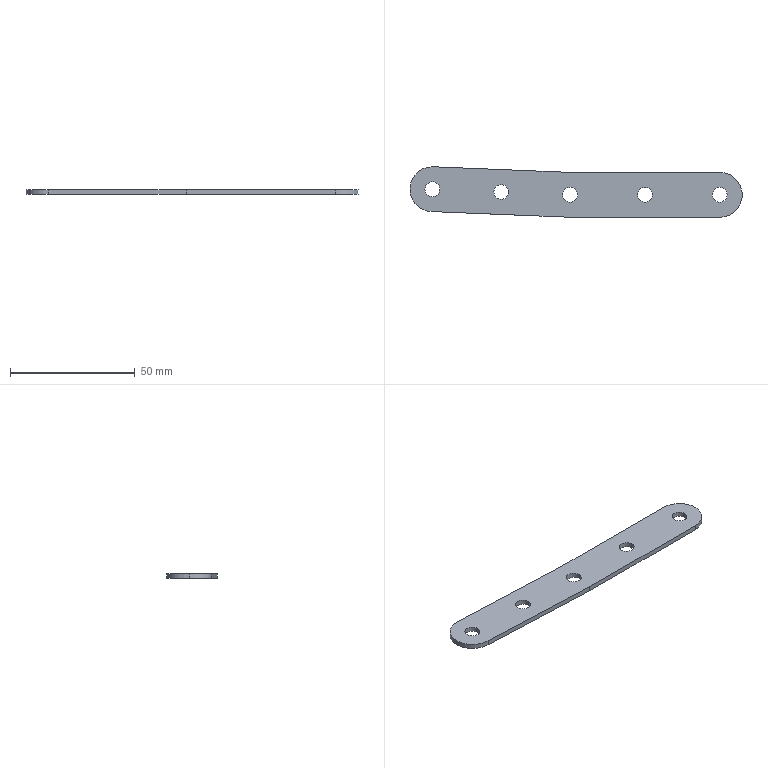Part | SolidWorks | features Extrusion 1 | 1 solid | 19 faces | box 133.234 x 20.271 x 2 mm | volume 4375 mm3 | cylinder 13 | plane 6 | commonest cylinder face diameters 6 x10 18 x3
STEP:
#1=CARTESIAN_POINT('',(82.234,-2.271,2.));
#2=VERTEX_POINT('',#1);
#3=CARTESIAN_POINT('',(88.234,-2.271,2.));
#4=VERTEX_POINT('',#3);
#5=CARTESIAN_POINT('',(85.234,-2.271,2.));
#6=DIRECTION('',(0.,0.,1.));
#7=DIRECTION('',(1.,0.,0.));
#8=AXIS2_PLACEMENT_3D('',#5,#6,#7);
#9=CIRCLE('',#8,3.);
#10=EDGE_CURVE('',#2,#4,#9,.T.);
#11=ORIENTED_EDGE('',*,*,#10,.T.);
#12=CARTESIAN_POINT('',(88.234,-2.271,0.));
#13=VERTEX_POINT('',#12);
#14=CARTESIAN_POINT('',(88.234,-2.271,2.));
#15=DIRECTION('',(0.,0.,-1.));
#16=VECTOR('',#15,1000.);
#17=LINE('',#14,#16);
#18=EDGE_CURVE('',#4,#13,#17,.T.);
#19=ORIENTED_EDGE('',*,*,#18,.T.);
#20=CARTESIAN_POINT('',(82.234,-2.271,0.));
#21=VERTEX_POINT('',#20);
#22=CARTESIAN_POINT('',(85.234,-2.271,0.));
#23=DIRECTION('',(0.,0.,1.));
#24=DIRECTION('',(1.,0.,0.));
#25=AXIS2_PLACEMENT_3D('',#22,#23,#24);
#26=CIRCLE('',#25,3.);
#27=EDGE_CURVE('',#21,#13,#26,.T.);
#28=ORIENTED_EDGE('',*,*,#27,.F.);
#29=CARTESIAN_POINT('',(82.234,-2.271,2.));
#30=DIRECTION('',(0.,0.,-1.));
#31=VECTOR('',#30,1000.);
#32=LINE('',#29,#31);
#33=EDGE_CURVE('',#2,#21,#32,.T.);
#34=ORIENTED_EDGE('',*,*,#33,.F.);
#35=EDGE_LOOP('',(#11,#19,#28,#34));
#36=FACE_OUTER_BOUND('',#35,.T.);
#37=CARTESIAN_POINT('',(85.234,-2.271,2.));
#38=DIRECTION('',(0.,0.,-1.));
#39=DIRECTION('',(-1.,0.,0.));
#40=AXIS2_PLACEMENT_3D('',#37,#38,#39);
#41=CYLINDRICAL_SURFACE('',#40,3.);
#42=ADVANCED_FACE('',(#36),#41,.F.);
#43=CARTESIAN_POINT('',(24.617,-1.136,2.));
#44=VERTEX_POINT('',#43);
#45=CARTESIAN_POINT('',(30.617,-1.136,2.));
#46=VERTEX_POINT('',#45);
#47=CARTESIAN_POINT('',(27.617,-1.136,2.));
#48=DIRECTION('',(0.,0.,1.));
#49=DIRECTION('',(1.,0.,0.));
#50=AXIS2_PLACEMENT_3D('',#47,#48,#49);
#51=CIRCLE('',#50,3.);
#52=EDGE_CURVE('',#44,#46,#51,.T.);
#53=ORIENTED_EDGE('',*,*,#52,.T.);
#54=CARTESIAN_POINT('',(30.617,-1.136,0.));
#55=VERTEX_POINT('',#54);
#56=CARTESIAN_POINT('',(30.617,-1.136,2.));
#57=DIRECTION('',(0.,0.,-1.));
#58=VECTOR('',#57,1000.);
#59=LINE('',#56,#58);
#60=EDGE_CURVE('',#46,#55,#59,.T.);
#61=ORIENTED_EDGE('',*,*,#60,.T.);
#62=CARTESIAN_POINT('',(24.617,-1.136,0.));
#63=VERTEX_POINT('',#62);
#64=CARTESIAN_POINT('',(27.617,-1.136,0.));
#65=DIRECTION('',(0.,0.,1.));
#66=DIRECTION('',(1.,0.,0.));
#67=AXIS2_PLACEMENT_3D('',#64,#65,#66);
#68=CIRCLE('',#67,3.);
#69=EDGE_CURVE('',#63,#55,#68,.T.);
#70=ORIENTED_EDGE('',*,*,#69,.F.);
#71=CARTESIAN_POINT('',(24.617,-1.136,2.));
#72=DIRECTION('',(0.,0.,-1.));
#73=VECTOR('',#72,1000.);
#74=LINE('',#71,#73);
#75=EDGE_CURVE('',#44,#63,#74,.T.);
#76=ORIENTED_EDGE('',*,*,#75,.F.);
#77=EDGE_LOOP('',(#53,#61,#70,#76));
#78=FACE_OUTER_BOUND('',#77,.T.);
#79=CARTESIAN_POINT('',(27.617,-1.136,2.));
#80=DIRECTION('',(0.,0.,-1.));
#81=DIRECTION('',(-1.,0.,0.));
#82=AXIS2_PLACEMENT_3D('',#79,#80,#81);
#83=CYLINDRICAL_SURFACE('',#82,3.);
#84=ADVANCED_FACE('',(#78),#83,.F.);
#85=CARTESIAN_POINT('',(112.234,-2.271,2.));
#86=VERTEX_POINT('',#85);
#87=CARTESIAN_POINT('',(118.234,-2.271,2.));
#88=VERTEX_POINT('',#87);
#89=CARTESIAN_POINT('',(115.234,-2.271,2.));
#90=DIRECTION('',(0.,0.,1.));
#91=DIRECTION('',(1.,0.,0.));
#92=AXIS2_PLACEMENT_3D('',#89,#90,#91);
#93=CIRCLE('',#92,3.);
#94=EDGE_CURVE('',#86,#88,#93,.T.);
#95=ORIENTED_EDGE('',*,*,#94,.T.);
#96=CARTESIAN_POINT('',(118.234,-2.271,0.));
#97=VERTEX_POINT('',#96);
#98=CARTESIAN_POINT('',(118.234,-2.271,2.));
#99=DIRECTION('',(0.,0.,-1.));
#100=VECTOR('',#99,1000.);
#101=LINE('',#98,#100);
#102=EDGE_CURVE('',#88,#97,#101,.T.);
#103=ORIENTED_EDGE('',*,*,#102,.T.);
#104=CARTESIAN_POINT('',(112.234,-2.271,0.));
#105=VERTEX_POINT('',#104);
#106=CARTESIAN_POINT('',(115.234,-2.271,0.));
#107=DIRECTION('',(0.,0.,1.));
#108=DIRECTION('',(1.,0.,0.));
#109=AXIS2_PLACEMENT_3D('',#106,#107,#108);
#110=CIRCLE('',#109,3.);
#111=EDGE_CURVE('',#105,#97,#110,.T.);
#112=ORIENTED_EDGE('',*,*,#111,.F.);
#113=CARTESIAN_POINT('',(112.234,-2.271,2.));
#114=DIRECTION('',(0.,0.,-1.));
#115=VECTOR('',#114,1000.);
#116=LINE('',#113,#115);
#117=EDGE_CURVE('',#86,#105,#116,.T.);
#118=ORIENTED_EDGE('',*,*,#117,.F.);
#119=EDGE_LOOP('',(#95,#103,#112,#118));
#120=FACE_OUTER_BOUND('',#119,.T.);
#121=CARTESIAN_POINT('',(115.234,-2.271,2.));
#122=DIRECTION('',(0.,0.,-1.));
#123=DIRECTION('',(-1.,0.,0.));
#124=AXIS2_PLACEMENT_3D('',#121,#122,#123);
#125=CYLINDRICAL_SURFACE('',#124,3.);
#126=ADVANCED_FACE('',(#120),#125,.F.);
#127=CARTESIAN_POINT('',(52.234,-2.271,2.));
#128=VERTEX_POINT('',#127);
#129=CARTESIAN_POINT('',(58.234,-2.271,2.));
#130=VERTEX_POINT('',#129);
#131=CARTESIAN_POINT('',(55.234,-2.271,2.));
#132=DIRECTION('',(0.,0.,1.));
#133=DIRECTION('',(1.,0.,0.));
#134=AXIS2_PLACEMENT_3D('',#131,#132,#133);
#135=CIRCLE('',#134,3.);
#136=EDGE_CURVE('',#128,#130,#135,.T.);
#137=ORIENTED_EDGE('',*,*,#136,.T.);
#138=CARTESIAN_POINT('',(58.234,-2.271,0.));
#139=VERTEX_POINT('',#138);
#140=CARTESIAN_POINT('',(58.234,-2.271,2.));
#141=DIRECTION('',(0.,0.,-1.));
#142=VECTOR('',#141,1000.);
#143=LINE('',#140,#142);
#144=EDGE_CURVE('',#130,#139,#143,.T.);
#145=ORIENTED_EDGE('',*,*,#144,.T.);
#146=CARTESIAN_POINT('',(52.234,-2.271,0.));
#147=VERTEX_POINT('',#146);
#148=CARTESIAN_POINT('',(55.234,-2.271,0.));
#149=DIRECTION('',(0.,0.,1.));
#150=DIRECTION('',(1.,0.,0.));
#151=AXIS2_PLACEMENT_3D('',#148,#149,#150);
#152=CIRCLE('',#151,3.);
#153=EDGE_CURVE('',#147,#139,#152,.T.);
#154=ORIENTED_EDGE('',*,*,#153,.F.);
#155=CARTESIAN_POINT('',(52.234,-2.271,2.));
#156=DIRECTION('',(0.,0.,-1.));
#157=VECTOR('',#156,1000.);
#158=LINE('',#155,#157);
#159=EDGE_CURVE('',#128,#147,#158,.T.);
#160=ORIENTED_EDGE('',*,*,#159,.F.);
#161=EDGE_LOOP('',(#137,#145,#154,#160));
#162=FACE_OUTER_BOUND('',#161,.T.);
#163=CARTESIAN_POINT('',(55.234,-2.271,2.));
#164=DIRECTION('',(0.,0.,-1.));
#165=DIRECTION('',(-1.,0.,0.));
#166=AXIS2_PLACEMENT_3D('',#163,#164,#165);
#167=CYLINDRICAL_SURFACE('',#166,3.);
#168=ADVANCED_FACE('',(#162),#167,.F.);
#169=CARTESIAN_POINT('',(-3.,0.,2.));
#170=VERTEX_POINT('',#169);
#171=CARTESIAN_POINT('',(3.,0.,2.));
#172=VERTEX_POINT('',#171);
#173=CARTESIAN_POINT('',(0.,0.,2.));
#174=DIRECTION('',(0.,0.,1.));
#175=DIRECTION('',(1.,0.,0.));
#176=AXIS2_PLACEMENT_3D('',#173,#174,#175);
#177=CIRCLE('',#176,3.);
#178=EDGE_CURVE('',#170,#172,#177,.T.);
#179=ORIENTED_EDGE('',*,*,#178,.T.);
#180=CARTESIAN_POINT('',(3.,0.,0.));
#181=VERTEX_POINT('',#180);
#182=CARTESIAN_POINT('',(3.,0.,2.));
#183=DIRECTION('',(0.,0.,-1.));
#184=VECTOR('',#183,1000.);
#185=LINE('',#182,#184);
#186=EDGE_CURVE('',#172,#181,#185,.T.);
#187=ORIENTED_EDGE('',*,*,#186,.T.);
#188=CARTESIAN_POINT('',(-3.,0.,0.));
#189=VERTEX_POINT('',#188);
#190=CARTESIAN_POINT('',(0.,0.,0.));
#191=DIRECTION('',(0.,0.,1.));
#192=DIRECTION('',(1.,0.,0.));
#193=AXIS2_PLACEMENT_3D('',#190,#191,#192);
#194=CIRCLE('',#193,3.);
#195=EDGE_CURVE('',#189,#181,#194,.T.);
#196=ORIENTED_EDGE('',*,*,#195,.F.);
#197=CARTESIAN_POINT('',(-3.,0.,2.));
#198=DIRECTION('',(0.,0.,-1.));
#199=VECTOR('',#198,1000.);
#200=LINE('',#197,#199);
#201=EDGE_CURVE('',#170,#189,#200,.T.);
#202=ORIENTED_EDGE('',*,*,#201,.F.);
#203=EDGE_LOOP('',(#179,#187,#196,#202));
#204=FACE_OUTER_BOUND('',#203,.T.);
#205=CARTESIAN_POINT('',(0.,0.,2.));
#206=DIRECTION('',(0.,0.,-1.));
#207=DIRECTION('',(-1.,0.,0.));
#208=AXIS2_PLACEMENT_3D('',#205,#206,#207);
#209=CYLINDRICAL_SURFACE('',#208,3.);
#210=ADVANCED_FACE('',(#204),#209,.F.);
#211=CARTESIAN_POINT('',(-9.,0.,2.));
#212=VERTEX_POINT('',#211);
#213=CARTESIAN_POINT('',(0.,-9.,2.));
#214=VERTEX_POINT('',#213);
#215=CARTESIAN_POINT('',(0.,0.,2.));
#216=DIRECTION('',(0.,0.,1.));
#217=DIRECTION('',(1.,0.,0.));
#218=AXIS2_PLACEMENT_3D('',#215,#216,#217);
#219=CIRCLE('',#218,9.);
#220=EDGE_CURVE('',#212,#214,#219,.T.);
#221=ORIENTED_EDGE('',*,*,#220,.F.);
#222=CARTESIAN_POINT('',(-9.,0.,0.));
#223=VERTEX_POINT('',#222);
#224=CARTESIAN_POINT('',(-9.,0.,2.));
#225=DIRECTION('',(0.,0.,-1.));
#226=VECTOR('',#225,1000.);
#227=LINE('',#224,#226);
#228=EDGE_CURVE('',#212,#223,#227,.T.);
#229=ORIENTED_EDGE('',*,*,#228,.T.);
#230=CARTESIAN_POINT('',(0.,-9.,0.));
#231=VERTEX_POINT('',#230);
#232=CARTESIAN_POINT('',(0.,0.,0.));
#233=DIRECTION('',(0.,0.,1.));
#234=DIRECTION('',(1.,0.,0.));
#235=AXIS2_PLACEMENT_3D('',#232,#233,#234);
#236=CIRCLE('',#235,9.);
#237=EDGE_CURVE('',#223,#231,#236,.T.);
#238=ORIENTED_EDGE('',*,*,#237,.T.);
#239=CARTESIAN_POINT('',(0.,-9.,2.));
#240=DIRECTION('',(0.,0.,-1.));
#241=VECTOR('',#240,1000.);
#242=LINE('',#239,#241);
#243=EDGE_CURVE('',#214,#231,#242,.T.);
#244=ORIENTED_EDGE('',*,*,#243,.F.);
#245=EDGE_LOOP('',(#221,#229,#238,#244));
#246=FACE_OUTER_BOUND('',#245,.T.);
#247=CARTESIAN_POINT('',(0.,0.,2.));
#248=DIRECTION('',(0.,0.,-1.));
#249=DIRECTION('',(-1.,0.,0.));
#250=AXIS2_PLACEMENT_3D('',#247,#248,#249);
#251=CYLINDRICAL_SURFACE('',#250,9.);
#252=ADVANCED_FACE('',(#246),#251,.T.);
#253=ORIENTED_EDGE('',*,*,#52,.F.);
#254=CARTESIAN_POINT('',(27.617,-1.136,2.));
#255=DIRECTION('',(0.,0.,1.));
#256=DIRECTION('',(1.,0.,0.));
#257=AXIS2_PLACEMENT_3D('',#254,#255,#256);
#258=CIRCLE('',#257,3.);
#259=EDGE_CURVE('',#46,#44,#258,.T.);
#260=ORIENTED_EDGE('',*,*,#259,.F.);
#261=EDGE_LOOP('',(#253,#260));
#262=FACE_BOUND('',#261,.T.);
#263=ORIENTED_EDGE('',*,*,#136,.F.);
#264=CARTESIAN_POINT('',(55.234,-2.271,2.));
#265=DIRECTION('',(0.,0.,1.));
#266=DIRECTION('',(1.,0.,0.));
#267=AXIS2_PLACEMENT_3D('',#264,#265,#266);
#268=CIRCLE('',#267,3.);
#269=EDGE_CURVE('',#130,#128,#268,.T.);
#270=ORIENTED_EDGE('',*,*,#269,.F.);
#271=EDGE_LOOP('',(#263,#270));
#272=FACE_BOUND('',#271,.T.);
#273=CARTESIAN_POINT('',(0.,9.,2.));
#274=VERTEX_POINT('',#273);
#275=CARTESIAN_POINT('',(0.,0.,2.));
#276=DIRECTION('',(0.,0.,1.));
#277=DIRECTION('',(1.,0.,0.));
#278=AXIS2_PLACEMENT_3D('',#275,#276,#277);
#279=CIRCLE('',#278,9.);
#280=EDGE_CURVE('',#274,#212,#279,.T.);
#281=ORIENTED_EDGE('',*,*,#280,.T.);
#282=ORIENTED_EDGE('',*,*,#220,.T.);
#283=CARTESIAN_POINT('',(55.234,-11.271,2.));
#284=VERTEX_POINT('',#283);
#285=CARTESIAN_POINT('',(0.,-9.,2.));
#286=DIRECTION('',(0.9992,-0.04109,0.));
#287=VECTOR('',#286,1000.);
#288=LINE('',#285,#287);
#289=EDGE_CURVE('',#214,#284,#288,.T.);
#290=ORIENTED_EDGE('',*,*,#289,.T.);
#291=CARTESIAN_POINT('',(115.234,-11.271,2.));
#292=VERTEX_POINT('',#291);
#293=CARTESIAN_POINT('',(55.234,-11.271,2.));
#294=DIRECTION('',(1.,0.,0.));
#295=VECTOR('',#294,1000.);
#296=LINE('',#293,#295);
#297=EDGE_CURVE('',#284,#292,#296,.T.);
#298=ORIENTED_EDGE('',*,*,#297,.T.);
#299=CARTESIAN_POINT('',(115.234,6.729,2.));
#300=VERTEX_POINT('',#299);
#301=CARTESIAN_POINT('',(115.234,-2.271,2.));
#302=DIRECTION('',(0.,0.,1.));
#303=DIRECTION('',(1.,0.,0.));
#304=AXIS2_PLACEMENT_3D('',#301,#302,#303);
#305=CIRCLE('',#304,9.);
#306=EDGE_CURVE('',#292,#300,#305,.T.);
#307=ORIENTED_EDGE('',*,*,#306,.T.);
#308=CARTESIAN_POINT('',(55.234,6.729,2.));
#309=VERTEX_POINT('',#308);
#310=CARTESIAN_POINT('',(55.234,6.729,2.));
#311=DIRECTION('',(-1.,0.,0.));
#312=VECTOR('',#311,1000.);
#313=LINE('',#310,#312);
#314=EDGE_CURVE('',#300,#309,#313,.T.);
#315=ORIENTED_EDGE('',*,*,#314,.T.);
#316=CARTESIAN_POINT('',(0.,9.,2.));
#317=DIRECTION('',(-0.9992,0.04109,0.));
#318=VECTOR('',#317,1000.);
#319=LINE('',#316,#318);
#320=EDGE_CURVE('',#309,#274,#319,.T.);
#321=ORIENTED_EDGE('',*,*,#320,.T.);
#322=EDGE_LOOP('',(#281,#282,#290,#298,#307,#315,#321));
#323=FACE_OUTER_BOUND('',#322,.T.);
#324=ORIENTED_EDGE('',*,*,#178,.F.);
#325=CARTESIAN_POINT('',(0.,0.,2.));
#326=DIRECTION('',(0.,0.,1.));
#327=DIRECTION('',(1.,0.,0.));
#328=AXIS2_PLACEMENT_3D('',#325,#326,#327);
#329=CIRCLE('',#328,3.);
#330=EDGE_CURVE('',#172,#170,#329,.T.);
#331=ORIENTED_EDGE('',*,*,#330,.F.);
#332=EDGE_LOOP('',(#324,#331));
#333=FACE_BOUND('',#332,.T.);
#334=ORIENTED_EDGE('',*,*,#94,.F.);
#335=CARTESIAN_POINT('',(115.234,-2.271,2.));
#336=DIRECTION('',(0.,0.,1.));
#337=DIRECTION('',(1.,0.,0.));
#338=AXIS2_PLACEMENT_3D('',#335,#336,#337);
#339=CIRCLE('',#338,3.);
#340=EDGE_CURVE('',#88,#86,#339,.T.);
#341=ORIENTED_EDGE('',*,*,#340,.F.);
#342=EDGE_LOOP('',(#334,#341));
#343=FACE_BOUND('',#342,.T.);
#344=ORIENTED_EDGE('',*,*,#10,.F.);
#345=CARTESIAN_POINT('',(85.234,-2.271,2.));
#346=DIRECTION('',(0.,0.,1.));
#347=DIRECTION('',(1.,0.,0.));
#348=AXIS2_PLACEMENT_3D('',#345,#346,#347);
#349=CIRCLE('',#348,3.);
#350=EDGE_CURVE('',#4,#2,#349,.T.);
#351=ORIENTED_EDGE('',*,*,#350,.F.);
#352=EDGE_LOOP('',(#344,#351));
#353=FACE_BOUND('',#352,.T.);
#354=CARTESIAN_POINT('',(0.,0.,2.));
#355=DIRECTION('',(0.,0.,1.));
#356=DIRECTION('',(1.,0.,0.));
#357=AXIS2_PLACEMENT_3D('',#354,#355,#356);
#358=PLANE('',#357);
#359=ADVANCED_FACE('',(#262,#272,#323,#333,#343,#353),#358,.T.);
#360=CARTESIAN_POINT('',(0.,9.,0.));
#361=VERTEX_POINT('',#360);
#362=CARTESIAN_POINT('',(0.,0.,0.));
#363=DIRECTION('',(0.,0.,1.));
#364=DIRECTION('',(1.,0.,0.));
#365=AXIS2_PLACEMENT_3D('',#362,#363,#364);
#366=CIRCLE('',#365,9.);
#367=EDGE_CURVE('',#361,#223,#366,.T.);
#368=ORIENTED_EDGE('',*,*,#367,.F.);
#369=CARTESIAN_POINT('',(55.234,6.729,0.));
#370=VERTEX_POINT('',#369);
#371=CARTESIAN_POINT('',(0.,9.,0.));
#372=DIRECTION('',(-0.9992,0.04109,0.));
#373=VECTOR('',#372,1000.);
#374=LINE('',#371,#373);
#375=EDGE_CURVE('',#370,#361,#374,.T.);
#376=ORIENTED_EDGE('',*,*,#375,.F.);
#377=CARTESIAN_POINT('',(115.234,6.729,0.));
#378=VERTEX_POINT('',#377);
#379=CARTESIAN_POINT('',(55.234,6.729,0.));
#380=DIRECTION('',(-1.,0.,0.));
#381=VECTOR('',#380,1000.);
#382=LINE('',#379,#381);
#383=EDGE_CURVE('',#378,#370,#382,.T.);
#384=ORIENTED_EDGE('',*,*,#383,.F.);
#385=CARTESIAN_POINT('',(115.234,-11.271,0.));
#386=VERTEX_POINT('',#385);
#387=CARTESIAN_POINT('',(115.234,-2.271,0.));
#388=DIRECTION('',(0.,0.,1.));
#389=DIRECTION('',(1.,0.,0.));
#390=AXIS2_PLACEMENT_3D('',#387,#388,#389);
#391=CIRCLE('',#390,9.);
#392=EDGE_CURVE('',#386,#378,#391,.T.);
#393=ORIENTED_EDGE('',*,*,#392,.F.);
#394=CARTESIAN_POINT('',(55.234,-11.271,0.));
#395=VERTEX_POINT('',#394);
#396=CARTESIAN_POINT('',(55.234,-11.271,0.));
#397=DIRECTION('',(1.,0.,0.));
#398=VECTOR('',#397,1000.);
#399=LINE('',#396,#398);
#400=EDGE_CURVE('',#395,#386,#399,.T.);
#401=ORIENTED_EDGE('',*,*,#400,.F.);
#402=CARTESIAN_POINT('',(0.,-9.,0.));
#403=DIRECTION('',(0.9992,-0.04109,0.));
#404=VECTOR('',#403,1000.);
#405=LINE('',#402,#404);
#406=EDGE_CURVE('',#231,#395,#405,.T.);
#407=ORIENTED_EDGE('',*,*,#406,.F.);
#408=ORIENTED_EDGE('',*,*,#237,.F.);
#409=EDGE_LOOP('',(#368,#376,#384,#393,#401,#407,#408));
#410=FACE_OUTER_BOUND('',#409,.T.);
#411=ORIENTED_EDGE('',*,*,#195,.T.);
#412=CARTESIAN_POINT('',(0.,0.,0.));
#413=DIRECTION('',(0.,0.,1.));
#414=DIRECTION('',(1.,0.,0.));
#415=AXIS2_PLACEMENT_3D('',#412,#413,#414);
#416=CIRCLE('',#415,3.);
#417=EDGE_CURVE('',#181,#189,#416,.T.);
#418=ORIENTED_EDGE('',*,*,#417,.T.);
#419=EDGE_LOOP('',(#411,#418));
#420=FACE_BOUND('',#419,.T.);
#421=ORIENTED_EDGE('',*,*,#153,.T.);
#422=CARTESIAN_POINT('',(55.234,-2.271,0.));
#423=DIRECTION('',(0.,0.,1.));
#424=DIRECTION('',(1.,0.,0.));
#425=AXIS2_PLACEMENT_3D('',#422,#423,#424);
#426=CIRCLE('',#425,3.);
#427=EDGE_CURVE('',#139,#147,#426,.T.);
#428=ORIENTED_EDGE('',*,*,#427,.T.);
#429=EDGE_LOOP('',(#421,#428));
#430=FACE_BOUND('',#429,.T.);
#431=ORIENTED_EDGE('',*,*,#111,.T.);
#432=CARTESIAN_POINT('',(115.234,-2.271,0.));
#433=DIRECTION('',(0.,0.,1.));
#434=DIRECTION('',(1.,0.,0.));
#435=AXIS2_PLACEMENT_3D('',#432,#433,#434);
#436=CIRCLE('',#435,3.);
#437=EDGE_CURVE('',#97,#105,#436,.T.);
#438=ORIENTED_EDGE('',*,*,#437,.T.);
#439=EDGE_LOOP('',(#431,#438));
#440=FACE_BOUND('',#439,.T.);
#441=ORIENTED_EDGE('',*,*,#69,.T.);
#442=CARTESIAN_POINT('',(27.617,-1.136,0.));
#443=DIRECTION('',(0.,0.,1.));
#444=DIRECTION('',(1.,0.,0.));
#445=AXIS2_PLACEMENT_3D('',#442,#443,#444);
#446=CIRCLE('',#445,3.);
#447=EDGE_CURVE('',#55,#63,#446,.T.);
#448=ORIENTED_EDGE('',*,*,#447,.T.);
#449=EDGE_LOOP('',(#441,#448));
#450=FACE_BOUND('',#449,.T.);
#451=ORIENTED_EDGE('',*,*,#27,.T.);
#452=CARTESIAN_POINT('',(85.234,-2.271,0.));
#453=DIRECTION('',(0.,0.,1.));
#454=DIRECTION('',(1.,0.,0.));
#455=AXIS2_PLACEMENT_3D('',#452,#453,#454);
#456=CIRCLE('',#455,3.);
#457=EDGE_CURVE('',#13,#21,#456,.T.);
#458=ORIENTED_EDGE('',*,*,#457,.T.);
#459=EDGE_LOOP('',(#451,#458));
#460=FACE_BOUND('',#459,.T.);
#461=CARTESIAN_POINT('',(0.,0.,0.));
#462=DIRECTION('',(0.,0.,1.));
#463=DIRECTION('',(1.,0.,0.));
#464=AXIS2_PLACEMENT_3D('',#461,#462,#463);
#465=PLANE('',#464);
#466=ADVANCED_FACE('',(#410,#420,#430,#440,#450,#460),#465,.F.);
#467=ORIENTED_EDGE('',*,*,#228,.F.);
#468=ORIENTED_EDGE('',*,*,#280,.F.);
#469=CARTESIAN_POINT('',(0.,9.,2.));
#470=DIRECTION('',(0.,0.,-1.));
#471=VECTOR('',#470,1000.);
#472=LINE('',#469,#471);
#473=EDGE_CURVE('',#274,#361,#472,.T.);
#474=ORIENTED_EDGE('',*,*,#473,.T.);
#475=ORIENTED_EDGE('',*,*,#367,.T.);
#476=EDGE_LOOP('',(#467,#468,#474,#475));
#477=FACE_OUTER_BOUND('',#476,.T.);
#478=CARTESIAN_POINT('',(0.,0.,2.));
#479=DIRECTION('',(0.,0.,-1.));
#480=DIRECTION('',(-1.,0.,0.));
#481=AXIS2_PLACEMENT_3D('',#478,#479,#480);
#482=CYLINDRICAL_SURFACE('',#481,9.);
#483=ADVANCED_FACE('',(#477),#482,.T.);
#484=ORIENTED_EDGE('',*,*,#406,.T.);
#485=CARTESIAN_POINT('',(55.234,-11.271,2.));
#486=DIRECTION('',(0.,0.,-1.));
#487=VECTOR('',#486,1000.);
#488=LINE('',#485,#487);
#489=EDGE_CURVE('',#284,#395,#488,.T.);
#490=ORIENTED_EDGE('',*,*,#489,.F.);
#491=ORIENTED_EDGE('',*,*,#289,.F.);
#492=ORIENTED_EDGE('',*,*,#243,.T.);
#493=EDGE_LOOP('',(#484,#490,#491,#492));
#494=FACE_OUTER_BOUND('',#493,.T.);
#495=CARTESIAN_POINT('',(0.,-9.,2.));
#496=DIRECTION('',(0.04109,0.9992,0.));
#497=DIRECTION('',(-0.9992,0.04109,0.));
#498=AXIS2_PLACEMENT_3D('',#495,#496,#497);
#499=PLANE('',#498);
#500=ADVANCED_FACE('',(#494),#499,.F.);
#501=ORIENTED_EDGE('',*,*,#400,.T.);
#502=CARTESIAN_POINT('',(115.234,-11.271,2.));
#503=DIRECTION('',(0.,0.,-1.));
#504=VECTOR('',#503,1000.);
#505=LINE('',#502,#504);
#506=EDGE_CURVE('',#292,#386,#505,.T.);
#507=ORIENTED_EDGE('',*,*,#506,.F.);
#508=ORIENTED_EDGE('',*,*,#297,.F.);
#509=ORIENTED_EDGE('',*,*,#489,.T.);
#510=EDGE_LOOP('',(#501,#507,#508,#509));
#511=FACE_OUTER_BOUND('',#510,.T.);
#512=CARTESIAN_POINT('',(55.234,-11.271,2.));
#513=DIRECTION('',(0.,1.,0.));
#514=DIRECTION('',(-1.,0.,0.));
#515=AXIS2_PLACEMENT_3D('',#512,#513,#514);
#516=PLANE('',#515);
#517=ADVANCED_FACE('',(#511),#516,.F.);
#518=ORIENTED_EDGE('',*,*,#392,.T.);
#519=CARTESIAN_POINT('',(115.234,6.729,2.));
#520=DIRECTION('',(0.,0.,-1.));
#521=VECTOR('',#520,1000.);
#522=LINE('',#519,#521);
#523=EDGE_CURVE('',#300,#378,#522,.T.);
#524=ORIENTED_EDGE('',*,*,#523,.F.);
#525=ORIENTED_EDGE('',*,*,#306,.F.);
#526=ORIENTED_EDGE('',*,*,#506,.T.);
#527=EDGE_LOOP('',(#518,#524,#525,#526));
#528=FACE_OUTER_BOUND('',#527,.T.);
#529=CARTESIAN_POINT('',(115.234,-2.271,2.));
#530=DIRECTION('',(0.,0.,-1.));
#531=DIRECTION('',(-1.,0.,0.));
#532=AXIS2_PLACEMENT_3D('',#529,#530,#531);
#533=CYLINDRICAL_SURFACE('',#532,9.);
#534=ADVANCED_FACE('',(#528),#533,.T.);
#535=ORIENTED_EDGE('',*,*,#383,.T.);
#536=CARTESIAN_POINT('',(55.234,6.729,2.));
#537=DIRECTION('',(0.,0.,-1.));
#538=VECTOR('',#537,1000.);
#539=LINE('',#536,#538);
#540=EDGE_CURVE('',#309,#370,#539,.T.);
#541=ORIENTED_EDGE('',*,*,#540,.F.);
#542=ORIENTED_EDGE('',*,*,#314,.F.);
#543=ORIENTED_EDGE('',*,*,#523,.T.);
#544=EDGE_LOOP('',(#535,#541,#542,#543));
#545=FACE_OUTER_BOUND('',#544,.T.);
#546=CARTESIAN_POINT('',(55.234,6.729,2.));
#547=DIRECTION('',(0.,-1.,0.));
#548=DIRECTION('',(1.,0.,0.));
#549=AXIS2_PLACEMENT_3D('',#546,#547,#548);
#550=PLANE('',#549);
#551=ADVANCED_FACE('',(#545),#550,.F.);
#552=ORIENTED_EDGE('',*,*,#375,.T.);
#553=ORIENTED_EDGE('',*,*,#473,.F.);
#554=ORIENTED_EDGE('',*,*,#320,.F.);
#555=ORIENTED_EDGE('',*,*,#540,.T.);
#556=EDGE_LOOP('',(#552,#553,#554,#555));
#557=FACE_OUTER_BOUND('',#556,.T.);
#558=CARTESIAN_POINT('',(0.,9.,2.));
#559=DIRECTION('',(-0.04109,-0.9992,0.));
#560=DIRECTION('',(0.9992,-0.04109,0.));
#561=AXIS2_PLACEMENT_3D('',#558,#559,#560);
#562=PLANE('',#561);
#563=ADVANCED_FACE('',(#557),#562,.F.);
#564=ORIENTED_EDGE('',*,*,#186,.F.);
#565=ORIENTED_EDGE('',*,*,#330,.T.);
#566=ORIENTED_EDGE('',*,*,#201,.T.);
#567=ORIENTED_EDGE('',*,*,#417,.F.);
#568=EDGE_LOOP('',(#564,#565,#566,#567));
#569=FACE_OUTER_BOUND('',#568,.T.);
#570=CARTESIAN_POINT('',(0.,0.,2.));
#571=DIRECTION('',(0.,0.,-1.));
#572=DIRECTION('',(-1.,0.,0.));
#573=AXIS2_PLACEMENT_3D('',#570,#571,#572);
#574=CYLINDRICAL_SURFACE('',#573,3.);
#575=ADVANCED_FACE('',(#569),#574,.F.);
#576=ORIENTED_EDGE('',*,*,#144,.F.);
#577=ORIENTED_EDGE('',*,*,#269,.T.);
#578=ORIENTED_EDGE('',*,*,#159,.T.);
#579=ORIENTED_EDGE('',*,*,#427,.F.);
#580=EDGE_LOOP('',(#576,#577,#578,#579));
#581=FACE_OUTER_BOUND('',#580,.T.);
#582=CARTESIAN_POINT('',(55.234,-2.271,2.));
#583=DIRECTION('',(0.,0.,-1.));
#584=DIRECTION('',(-1.,0.,0.));
#585=AXIS2_PLACEMENT_3D('',#582,#583,#584);
#586=CYLINDRICAL_SURFACE('',#585,3.);
#587=ADVANCED_FACE('',(#581),#586,.F.);
#588=ORIENTED_EDGE('',*,*,#102,.F.);
#589=ORIENTED_EDGE('',*,*,#340,.T.);
#590=ORIENTED_EDGE('',*,*,#117,.T.);
#591=ORIENTED_EDGE('',*,*,#437,.F.);
#592=EDGE_LOOP('',(#588,#589,#590,#591));
#593=FACE_OUTER_BOUND('',#592,.T.);
#594=CARTESIAN_POINT('',(115.234,-2.271,2.));
#595=DIRECTION('',(0.,0.,-1.));
#596=DIRECTION('',(-1.,0.,0.));
#597=AXIS2_PLACEMENT_3D('',#594,#595,#596);
#598=CYLINDRICAL_SURFACE('',#597,3.);
#599=ADVANCED_FACE('',(#593),#598,.F.);
#600=ORIENTED_EDGE('',*,*,#60,.F.);
#601=ORIENTED_EDGE('',*,*,#259,.T.);
#602=ORIENTED_EDGE('',*,*,#75,.T.);
#603=ORIENTED_EDGE('',*,*,#447,.F.);
#604=EDGE_LOOP('',(#600,#601,#602,#603));
#605=FACE_OUTER_BOUND('',#604,.T.);
#606=CARTESIAN_POINT('',(27.617,-1.136,2.));
#607=DIRECTION('',(0.,0.,-1.));
#608=DIRECTION('',(-1.,0.,0.));
#609=AXIS2_PLACEMENT_3D('',#606,#607,#608);
#610=CYLINDRICAL_SURFACE('',#609,3.);
#611=ADVANCED_FACE('',(#605),#610,.F.);
#612=ORIENTED_EDGE('',*,*,#18,.F.);
#613=ORIENTED_EDGE('',*,*,#350,.T.);
#614=ORIENTED_EDGE('',*,*,#33,.T.);
#615=ORIENTED_EDGE('',*,*,#457,.F.);
#616=EDGE_LOOP('',(#612,#613,#614,#615));
#617=FACE_OUTER_BOUND('',#616,.T.);
#618=CARTESIAN_POINT('',(85.234,-2.271,2.));
#619=DIRECTION('',(0.,0.,-1.));
#620=DIRECTION('',(-1.,0.,0.));
#621=AXIS2_PLACEMENT_3D('',#618,#619,#620);
#622=CYLINDRICAL_SURFACE('',#621,3.);
#623=ADVANCED_FACE('',(#617),#622,.F.);
#624=CLOSED_SHELL('',(#42,#84,#126,#168,#210,#252,#359,#466,#483,#500,#517,#534,#551,#563,#575,#587,#599,#611,#623));
#625=MANIFOLD_SOLID_BREP('',#624);
#626=CARTESIAN_POINT('',(0.,0.,0.));
#627=DIRECTION('',(0.,0.,1.));
#628=DIRECTION('',(1.,0.,0.));
#629=AXIS2_PLACEMENT_3D('',#626,#627,#628);
#630=(LENGTH_UNIT()NAMED_UNIT(*)SI_UNIT(.MILLI.,.METRE.));
#631=UNCERTAINTY_MEASURE_WITH_UNIT(LENGTH_MEASURE(0.00001),#630,'','');
#632=(NAMED_UNIT(*)PLANE_ANGLE_UNIT()SI_UNIT($,.RADIAN.));
#633=(NAMED_UNIT(*)SI_UNIT($,.STERADIAN.)SOLID_ANGLE_UNIT());
#634=(GEOMETRIC_REPRESENTATION_CONTEXT(3)GLOBAL_UNCERTAINTY_ASSIGNED_CONTEXT((#631))GLOBAL_UNIT_ASSIGNED_CONTEXT((#630,#632,#633))REPRESENTATION_CONTEXT('',''));
#635=ADVANCED_BREP_SHAPE_REPRESENTATION('',(#625,#629),#634);